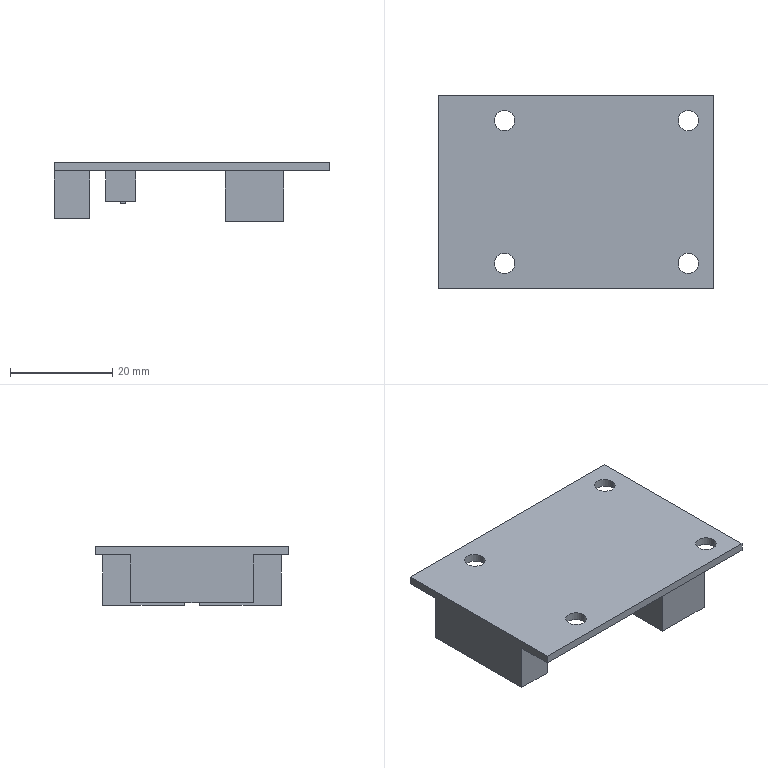Part | STEP file | Circuit board assembly | 1 solid | 83 faces | box 54 x 38 x 11.5 mm | volume 8666 mm3 | plane 75 | cylinder 8 | commonest cylinder face diameters 4 x8